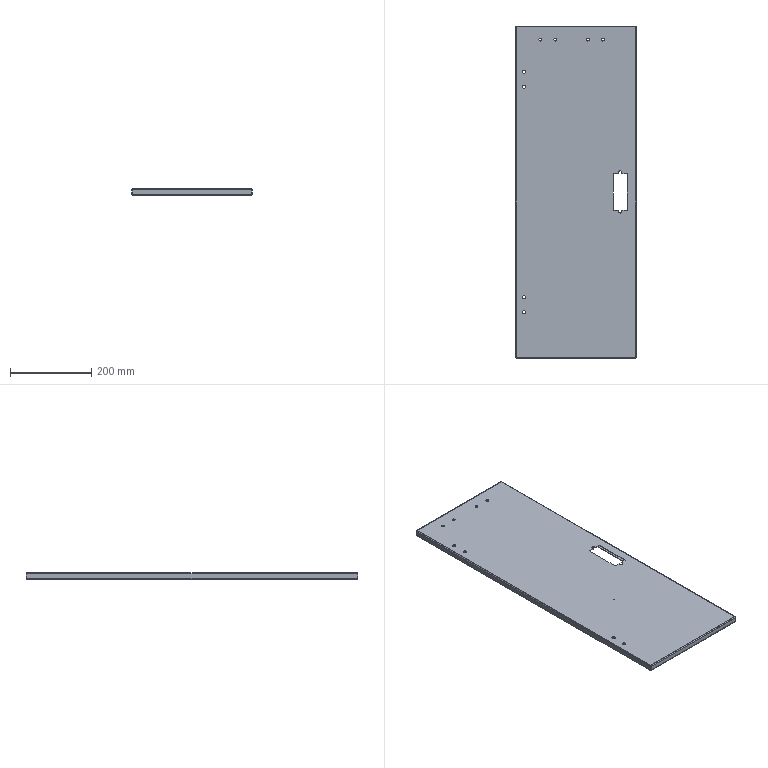Part | STEP file | 09-11 upper door B (Default) | 1 solid | 101 faces | box 298 x 818 x 15 mm | volume 444679 mm3 | plane 49 | cylinder 36 | spline 16 | commonest cylinder face diameters 8 x10 1.473 x8 4.473 x8 7 x8 4 x2